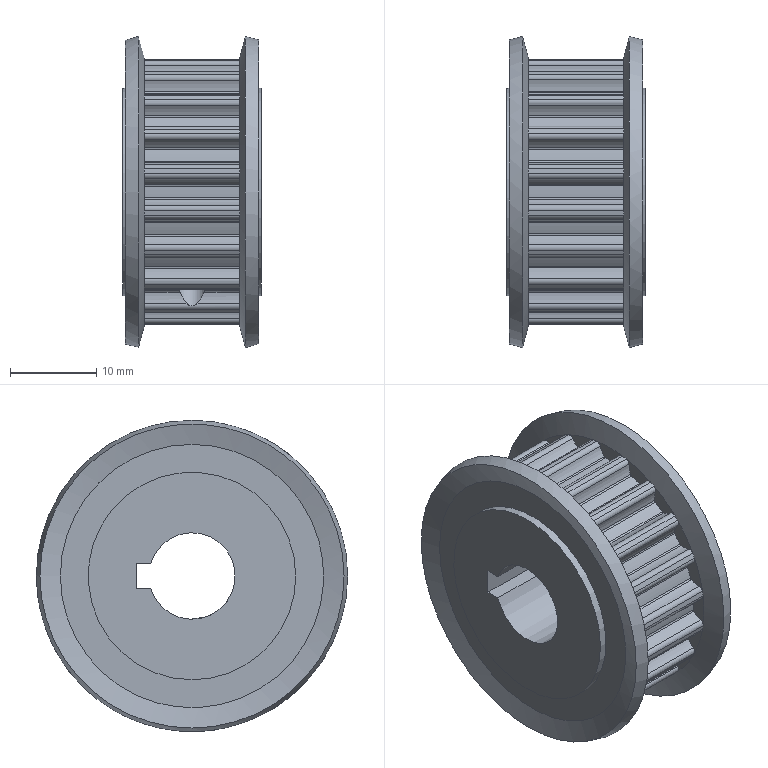Part | STEP file | C-HTPA20S5M100-A-N10 | 1 solid | 231 faces | box 16 x 36 x 36 mm | volume 9752 mm3 | cylinder 175 | plane 50 | cone 6 | commonest cylinder face diameters 0.5 x44 6.55 x44 1.1 x40 27.33 x22 30.87 x20 3.242 x2